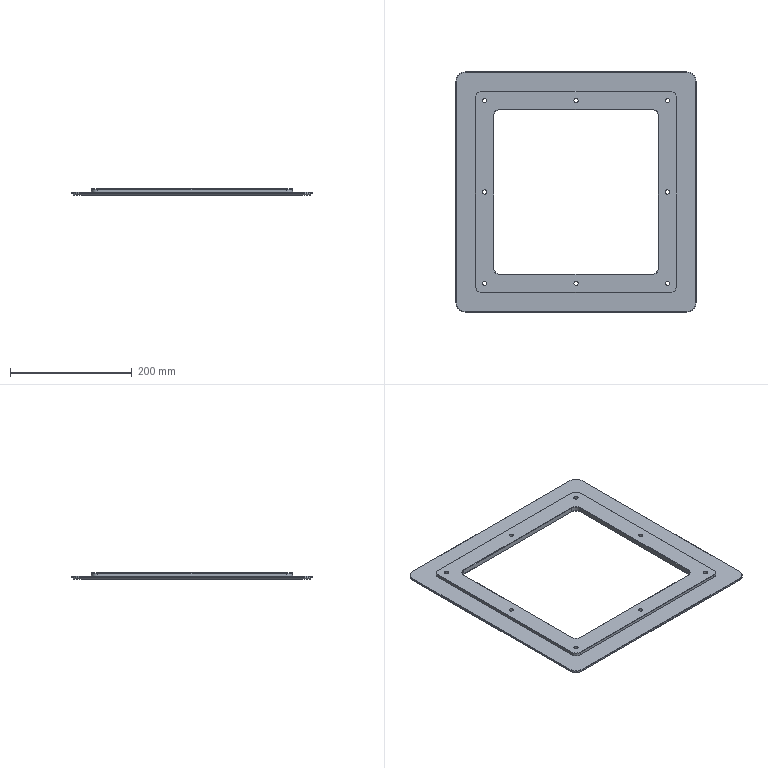NC program | Mastercam | posted with a generic post
Lines 4680 to 5147 of 5147:
N7210 T24 M6
N7220 G0 G90 G17 G54 X-251. Y157. A0. S1000 M3
N7230 G43 H24 Z50. M8
N7240 Z1.
N7250 G1 Z0. F600.
N7260 X-125. F300.
N7270 X125.
N7280 G2 X157. Y125. I0. J-32.
N7290 G1 Y-125.
N7300 G2 X125. Y-157. I-32. J0.
N7310 G1 X-125.
N7320 G2 X-157. Y-125. I0. J32.
N7330 G1 Y125.
N7340 G2 X-125. Y157. I32. J0.
N7350 G1 X1.
N7360 G0 Z50.
N7370 M5
N7380 G91 G28 Z0. M9
N7390 A0.
N7400 M01
N7410 T12 M6
N7420 G0 G90 G17 G54 X-176.504 Y-203.599 A0. S2000 M3
N7430 G43 H12 Z50. M8
N7440 Z-4.
N7450 G1 Z-5. F600.
N7460 G3 X-176.525 Y-203.435 I-1.235 J-.072 F800.
N7470 X-176.567 Y-203.274 I-1.214 J-.236
N7480 X-176.631 Y-203.12 I-1.172 J-.397
N7490 X-176.715 Y-202.977 I-1.108 J-.551
N7500 X-176.817 Y-202.846 I-1.024 J-.694
N7510 X-176.936 Y-202.73 I-.922 J-.825
N7520 X-177.069 Y-202.63 I-.803 J-.941
N7530 X-177.215 Y-202.55 I-.67 J-1.041
N7540 G2 X-202.55 Y-177.206 I22.265 J47.592
N7550 G3 X-202.63 Y-177.061 I-1.121 J-.524
N7560 X-202.73 Y-176.927 I-1.041 J-.669
N7570 X-202.846 Y-176.808 I-.941 J-.803
N7580 X-202.977 Y-176.706 I-.825 J-.922
N7590 X-203.12 Y-176.622 I-.694 J-1.024
N7600 X-203.274 Y-176.558 I-.551 J-1.108
N7610 X-203.435 Y-176.515 I-.397 J-1.172
N7620 X-203.599 Y-176.495 I-.236 J-1.215
N7630 G0 Z50.
N7640 Y176.508
N7650 Z-4.
N7660 G1 Z-5. F600.
N7670 G3 X-203.435 Y176.528 I-.072 J1.235 F800.
N7680 X-203.274 Y176.571 I-.236 J1.215
N7690 X-203.12 Y176.635 I-.397 J1.172
N7700 X-202.977 Y176.719 I-.551 J1.108
N7710 X-202.846 Y176.821 I-.694 J1.024
N7720 X-202.73 Y176.94 I-.825 J.922
N7730 X-202.63 Y177.073 I-.941 J.803
N7740 X-202.55 Y177.219 I-1.041 J.67
N7750 G2 X-177.21 Y202.55 I47.588 J-22.265
N7760 G3 X-177.065 Y202.63 I-.524 J1.121
N7770 X-176.931 Y202.73 I-.669 J1.041
N7780 X-176.812 Y202.846 I-.803 J.941
N7790 X-176.71 Y202.977 I-.922 J.825
N7800 X-176.626 Y203.12 I-1.024 J.694
N7810 X-176.562 Y203.274 I-1.108 J.551
N7820 X-176.52 Y203.435 I-1.172 J.397
N7830 X-176.499 Y203.599 I-1.214 J.236
N7840 G0 Z50.
N7850 X176.508
N7860 Z-4.
N7870 G1 Z-5. F600.
N7880 G3 X176.528 Y203.435 I1.235 J.072 F800.
N7890 X176.571 Y203.274 I1.215 J.236
N7900 X176.635 Y203.12 I1.172 J.397
N7910 X176.719 Y202.977 I1.108 J.551
N7920 X176.821 Y202.846 I1.024 J.694
N7930 X176.94 Y202.73 I.922 J.825
N7940 X177.073 Y202.63 I.803 J.941
N7950 X177.219 Y202.55 I.67 J1.041
N7960 G2 X202.55 Y177.21 I-22.265 J-47.588
N7970 G3 X202.63 Y177.065 I1.121 J.524
N7980 X202.73 Y176.931 I1.041 J.669
N7990 X202.846 Y176.812 I.941 J.803
N8000 X202.977 Y176.71 I.825 J.922
N8010 X203.12 Y176.626 I.694 J1.024
N8020 X203.274 Y176.562 I.551 J1.108
N8030 X203.435 Y176.52 I.397 J1.172
N8040 X203.599 Y176.499 I.236 J1.214
N8050 G0 Z50.
N8060 Y-176.508
N8070 Z-4.
N8080 G1 Z-5. F600.
N8090 G3 X203.435 Y-176.528 I.072 J-1.235 F800.
N8100 X203.274 Y-176.571 I.236 J-1.215
N8110 X203.12 Y-176.635 I.397 J-1.172
N8120 X202.977 Y-176.719 I.551 J-1.108
N8130 X202.846 Y-176.821 I.694 J-1.024
N8140 X202.73 Y-176.94 I.825 J-.922
N8150 X202.63 Y-177.073 I.941 J-.803
N8160 X202.55 Y-177.219 I1.041 J-.67
N8170 G2 X177.21 Y-202.55 I-47.588 J22.265
N8180 X176.686 Y-202.666 I-.524 J1.121
N8190 X175.685 Y-202.156 I0. J1.237
N8200 G1 X171.401 Y-196.259
N8210 G3 X170.4 Y-195.749 I-1.001 J-.727
N8220 X169.973 Y-195.824 I0. J-1.237
N8230 G2 X160.921 Y-198.084 I-15.013 J40.871
N8240 X154.569 Y-198.499 I-6.837 J55.808
N8250 G1 X-154.569
N8260 G2 X-154.947 Y-198.501 I-.378 J43.546
N8270 X-197.374 Y-164.771 I0. J43.548
N8280 X-198.497 Y-154.911 I57.043 J11.49
N8290 G1 X-198.499 Y0.
N8300 Y154.569
N8310 G2 X-198.501 Y154.953 I43.539 J.384
N8320 X-160.921 Y198.084 I43.541 J0.
N8330 X-154.569 Y198.499 I6.837 J-55.808
N8340 G1 X154.569
N8350 G2 X154.953 Y198.501 I.384 J-43.539
N8360 X198.084 Y160.921 I0. J-43.541
N8370 X198.499 Y154.569 I-55.808 J-6.837
N8380 G1 Y-154.569
N8390 G2 X198.501 Y-154.953 I-43.539 J-.384
N8400 X169.973 Y-195.824 I-43.541 J0.
N8410 X169.546 Y-195.9 I-.427 J1.161
N8420 X168.488 Y-195.304 I0. J1.237
N8430 G1 X164.681 Y-189.022
N8440 G3 X163.623 Y-188.426 I-1.058 J-.642
N8450 X163.324 Y-188.463 I0. J-1.238
N8460 G2 X158.096 Y-189.347 I-8.353 J33.505
N8470 G1 X154.797 Y-189.498
N8480 X-154.569 Y-189.5
N8490 G2 X-154.953 Y-189.502 I-.384 J34.532
N8500 X-188.925 Y-161.172 I0. J34.534
N8510 X-189.5 Y-154.569 I40.729 J6.872
N8520 G1 Y0.
N8530 Y154.569
N8540 G2 X-189.502 Y154.958 I34.529 J.389
N8550 X-158.096 Y189.347 I34.531 J0.
N8560 G1 X-154.797 Y189.498
N8570 X154.569 Y189.5
N8580 G2 X154.958 Y189.502 I.389 J-34.529
N8590 X189.347 Y158.096 I0. J-34.531
N8600 G1 X189.498 Y154.797
N8610 X189.5 Y-154.569
N8620 G2 X189.502 Y-154.958 I-34.529 J-.389
N8630 X163.324 Y-188.463 I-34.531 J0.
N8640 X163.024 Y-188.5 I-.3 J1.201
N8650 X161.909 Y-187.8 I0. J1.238
N8660 G1 X158.663 Y-181.066
N8670 G3 X157.549 Y-180.367 I-1.114 J-.538
N8680 G1 X157.491 Y-180.368
N8690 X154.683 Y-180.499
N8700 X-154.569 Y-180.5
N8710 G2 X-154.948 Y-180.503 I-.379 J25.548
N8720 X-180.287 Y-158.232 I0. J25.551
N8730 X-180.5 Y-154.569 I32.125 J3.707
N8740 G1 Y0.
N8750 Y154.569
N8760 G2 X-180.503 Y154.953 I25.538 J.384
N8770 X-157.492 Y180.367 I25.541 J0.
N8780 G1 X-154.683 Y180.499
N8790 X154.569 Y180.5
N8800 G2 X154.953 Y180.503 I.384 J-25.538
N8810 X180.367 Y157.492 I0. J-25.541
N8820 G1 X180.499 Y154.683
N8830 X180.5 Y-154.569
N8840 G2 X180.503 Y-154.953 I-25.538 J-.384
N8850 X157.492 Y-180.367 I-25.541 J0.
N8860 X157.433 Y-180.368 I-.059 J1.236
N8870 X156.249 Y-179.492 I0. J1.237
N8880 G1 X154.078 Y-172.376
N8890 G3 X152.894 Y-171.5 I-1.184 J-.362
N8900 G1 X-154.569
N8910 G2 X-154.892 Y-171.503 I-.323 J16.746
N8920 X-165.389 Y-167.805 I0. J16.749
N8930 X-171.388 Y-156.888 I10.437 J12.842
N8940 X-171.5 Y-154.569 I47.948 J3.482
N8950 G1 Y0.
N8960 Y154.569
N8970 G2 X-171.503 Y154.9 I16.709 J.331
N8980 X-166.935 Y166.381 I16.712 J0.
N8990 X-155.342 Y171.49 I11.962 J-11.435
N9000 G1 X-154.569 Y171.5
N9010 X154.569
N9020 G2 X154.9 Y171.503 I.331 J-16.709
N9030 X166.381 Y166.935 I0. J-16.712
N9040 X171.49 Y155.342 I-11.435 J-11.962
N9050 G1 X171.5 Y154.569
N9060 Y-154.569
N9070 G2 X171.503 Y-154.9 I-16.709 J-.331
N9080 X166.935 Y-166.381 I-16.712 J0.
N9090 X155.342 Y-171.49 I-11.962 J11.435
N9100 G1 X154.569 Y-171.5
N9110 X152.894
N9120 G0 Z50.
N9130 X-168.859 Y167.162
N9140 Z-4.
N9150 G1 Z-5. F600.
N9160 X-168.011 Y166.314 F800.
N9170 G3 X-167.162 Y165.962 I.849 J.848
N9180 X-166.314 Y166.314 I0. J1.2
N9190 G2 X-155. Y171. I11.314 J-11.314
N9200 G1 X155.
N9210 G2 X171. Y155. I0. J-16.
N9220 G1 Y-155.
N9230 G2 X155. Y-171. I-16. J0.
N9240 G1 X-155.
N9250 G2 X-171. Y-155. I0. J16.
N9260 G1 Y155.
N9270 G2 X-166.314 Y166.314 I16. J0.
N9280 G3 X-165.963 Y167.162 I-.848 J.848
N9290 X-166.314 Y168.011 I-1.199 J0.
N9300 G1 X-167.162 Y168.859
N9310 X-168.859 Y167.162
N9320 X-168.011 Y166.314
N9330 G3 X-167.162 Y165.962 I.849 J.848
N9340 X-166.314 Y166.314 I0. J1.2
N9350 G2 X-155. Y171. I11.314 J-11.314
N9360 G1 X155.
N9370 G2 X171. Y155. I0. J-16.
N9380 G1 Y-155.
N9390 G2 X155. Y-171. I-16. J0.
N9400 G1 X-155.
N9410 G2 X-171. Y-155. I0. J16.
N9420 G1 Y155.
N9430 G2 X-166.314 Y166.314 I16. J0.
N9440 G3 X-165.963 Y167.162 I-.848 J.848
N9450 X-166.314 Y168.011 I-1.199 J0.
N9460 G1 X-167.162 Y168.859
N9470 G0 Z50.
N9480 M5
N9490 G91 G28 Z0. M9
N9500 A0.
N9510 M01
N9520 T7 M6
N9530 G0 G90 G17 G54 X-167.65 Y154. A0. S3500 M3
N9540 G43 H7 Z50. M8
N9550 Z.5
N9560 G1 Z-1. F600.
N9570 X-166.65 F500.
N9580 G3 X-165.65 Y155. I0. J1.
N9590 G2 X-155. Y165.65 I10.65 J0.
N9600 G1 X155.
N9610 G2 X165.65 Y155. I0. J-10.65
N9620 G1 Y-155.
N9630 G2 X155. Y-165.65 I-10.65 J0.
N9640 G1 X-155.
N9650 G2 X-165.65 Y-155. I0. J10.65
N9660 G1 Y155.
N9670 G3 X-166.65 Y156. I-1. J0.
N9680 G1 X-167.65
N9690 G0 Z50.
N9700 X-199.65 Y181.
N9710 Z-4.5
N9720 G1 Z-6. F600.
N9730 X-198.65 F500.
N9740 G3 X-197.65 Y182. I0. J1.
N9750 G2 X-182. Y197.65 I15.65 J0.
N9760 G1 X182.
N9770 G2 X197.65 Y182. I0. J-15.65
N9780 G1 Y-182.
N9790 G2 X182. Y-197.65 I-15.65 J0.
N9800 G1 X-182.
N9810 G2 X-197.65 Y-182. I0. J15.65
N9820 G1 Y182.
N9830 G3 X-198.65 Y183. I-1. J0.
N9840 G1 X-199.65
N9850 G0 Z50.
N9860 X-124. Y132.35
N9870 Z.5
N9880 G1 Z-1. F600.
N9890 Y133.35 F500.
N9900 G3 X-125. Y134.35 I-1. J0.
N9910 X-134.35 Y125. I0. J-9.35
N9920 G1 Y-125.
N9930 G3 X-125. Y-134.35 I9.35 J0.
N9940 G1 X125.
N9950 G3 X134.35 Y-125. I0. J9.35
N9960 G1 Y125.
N9970 G3 X125. Y134.35 I-9.35 J0.
N9980 G1 X-125.
N9990 G3 X-126. Y133.35 I0. J-1.
N100 G1 Y132.35
N110 G0 Z50.
N120 M5
N130 G91 G28 Z0. M9
N140 A0.
N150 M01
( OU )
N160 T14 M6
N170 G0 G90 G17 G54 X-124.8 Y124.8 A0. S1600 M3
N180 G43 H14 Z50. M8
N190 Z1.
N200 G1 Z0. F600.
N210 Y-124.8 Z-.075 F3000.
N220 X124.8 Z-.15
N230 Y124.8 Z-.225
N240 X-124.8 Z-.3
N250 Y-124.8 Z-.375
N260 X124.8 Z-.45
N270 Y124.8 Z-.525
N280 X-124.8 Z-.6
N290 Y-124.8 Z-.675
N300 X124.8 Z-.75
N310 Y124.8 Z-.825
N320 X-124.8 Z-.9
N330 Y-124.8 Z-.975
N340 X124.8 Z-1.05
N350 Y124.8 Z-1.125
N360 X-124.8 Z-1.2
N370 Y-124.8 Z-1.275
N380 X124.8 Z-1.35
N390 Y124.8 Z-1.425
N400 X-124.8 Z-1.5
N410 Y-124.8 Z-1.575
N420 X124.8 Z-1.65
N430 Y124.8 Z-1.725
N440 X-124.8 Z-1.8
N450 Y-124.8 Z-1.875
N460 X124.8 Z-1.95
N470 Y124.8 Z-2.025
N480 X-124.8 Z-2.1
N490 Y-124.8 Z-2.175
N500 X124.8 Z-2.25
N510 Y124.8 Z-2.325
N520 X-124.8 Z-2.4
N530 Y-124.8 Z-2.475
N540 X124.8 Z-2.55
N550 Y124.8 Z-2.625
N560 X-124.8 Z-2.7
N570 Y-124.8 Z-2.775
N580 X124.8 Z-2.85
N590 Y124.8 Z-2.925
N600 X-124.8 Z-3.
N610 Y-124.8 Z-3.075
N620 X124.8 Z-3.15
N630 Y124.8 Z-3.225
N640 X-124.8 Z-3.3
N650 Y-124.8 Z-3.375
N660 X124.8 Z-3.45
N670 Y124.8 Z-3.525
N680 X-124.8 Z-3.6
N690 Y-124.8 Z-3.675
N700 X124.8 Z-3.75
N710 Y124.8 Z-3.825
N720 X-124.8 Z-3.9
N730 Y-124.8 Z-3.975
N740 X124.8 Z-4.05
N750 Y124.8 Z-4.125
N760 X-124.8 Z-4.2
N770 Y-124.8 Z-4.275
N780 X124.8 Z-4.35
N790 Y124.8 Z-4.425
N800 X-124.8 Z-4.5
N810 Y-124.8 Z-4.575
N820 X124.8 Z-4.65
N830 Y124.8 Z-4.725
N840 X-124.8 Z-4.8
N850 Y-124.8 Z-4.875
N860 X124.8 Z-4.95
N870 Y124.8 Z-5.025
N880 X-124.8 Z-5.1
N890 Y-124.8 Z-5.175
N900 X124.8 Z-5.25
N910 Y124.8 Z-5.325
N920 X-124.8 Z-5.4
N930 Y-124.8 Z-5.475
N940 X124.8 Z-5.55
N950 Y124.8 Z-5.625
N960 X-124.8 Z-5.7
N970 Y-124.8 Z-5.775
N980 X124.8 Z-5.85
N990 Y124.8 Z-5.925
N1000 X-124.8 Z-6.
N1010 Y-124.8 Z-6.075
N1020 X124.8 Z-6.15
N1030 Y124.8 Z-6.225
N1040 X-124.8 Z-6.3
N1050 Y-124.8 Z-6.375
N1060 X124.8 Z-6.45
N1070 Y124.8 Z-6.525
N1080 X-124.8 Z-6.6
N1090 Y-124.8 Z-6.675
N1100 X124.8 Z-6.75
N1110 Y124.8 Z-6.825
N1120 X-124.8 Z-6.9
N1130 Y-124.8 Z-6.975
N1140 X124.8 Z-7.05
N1150 Y124.8 Z-7.125
N1160 X-124.8 Z-7.2
N1170 Y-124.8 Z-7.275
N1180 X124.8 Z-7.35
N1190 Y124.8 Z-7.425
N1200 X-124.8 Z-7.5
N1210 Y-124.8 Z-7.575
N1220 X124.8 Z-7.65
N1230 Y124.8 Z-7.725
N1240 X-124.8 Z-7.8
N1250 Y-124.8 Z-7.875
N1260 X124.8 Z-7.95
N1270 Y124.8 Z-8.025
N1280 X-124.8 Z-8.1
N1290 Y-124.8 Z-8.175
N1300 X124.8 Z-8.25
N1310 Y124.8 Z-8.325
N1320 X-124.8 Z-8.4
N1330 Y-124.8 Z-8.475
N1340 X124.8 Z-8.55
N1350 Y124.8 Z-8.625
N1360 X-124.8 Z-8.7
N1370 Y-124.8 Z-8.775
N1380 X124.8 Z-8.85
N1390 Y124.8 Z-8.925
N1400 X-124.8 Z-9.
N1410 Y-124.8 Z-9.075
N1420 X124.8 Z-9.15
N1430 Y124.8 Z-9.225
N1440 X-124.8 Z-9.3
N1450 Y-124.8 Z-9.375
N1460 X124.8 Z-9.45
N1470 Y124.8 Z-9.525
N1480 X-124.8 Z-9.6
N1490 Y-124.8 Z-9.675
N1500 X124.8 Z-9.75
N1510 Y124.8 Z-9.825
N1520 X-124.8 Z-9.9
N1530 Y-124.8
N1540 X124.8
N1550 Y124.8
N1560 X-124.8
N1570 G0 Z50.
N1580 M5
N1590 G91 G28 Z0. M9
N1600 A0.
N1610 M01
N1620 T12 M6
N1630 G0 G90 G17 G54 X-123.8 Y126.6 A0. S2000 M3
N1640 G43 H12 Z50. M8
N1650 Z1.
N1660 G1 Z-9.9 F600.
N1670 Y127.8 F800.
N1680 G3 X-125. Y129. I-1.2 J0.
N1690 X-129. Y125. I0. J-4.
N1700 G1 Y-125.
N1710 G3 X-125. Y-129. I4. J0.
N1720 G1 X125.
N1730 G3 X129. Y-125. I0. J4.
N1740 G1 Y125.
N1750 G3 X125. Y129. I-4. J0.
N1760 G1 X-125.
N1770 G3 X-126.2 Y127.8 I0. J-1.2
N1780 G1 Y126.6
N1790 X-123.8
N1800 Y127.8
N1810 G3 X-125. Y129. I-1.2 J0.
N1820 X-129. Y125. I0. J-4.
N1830 G1 Y-125.
N1840 G3 X-125. Y-129. I4. J0.
N1850 G1 X125.
N1860 G3 X129. Y-125. I0. J4.
N1870 G1 Y125.
N1880 G3 X125. Y129. I-4. J0.
N1890 G1 X-125.
N1900 G3 X-126.2 Y127.8 I0. J-1.2
N1910 G1 Y126.6
N1920 G0 Z50.
N1930 M5
N1940 G91 G28 Z0. M9
N1950 G28 X0. Y0. A0.
N1960 M30
%